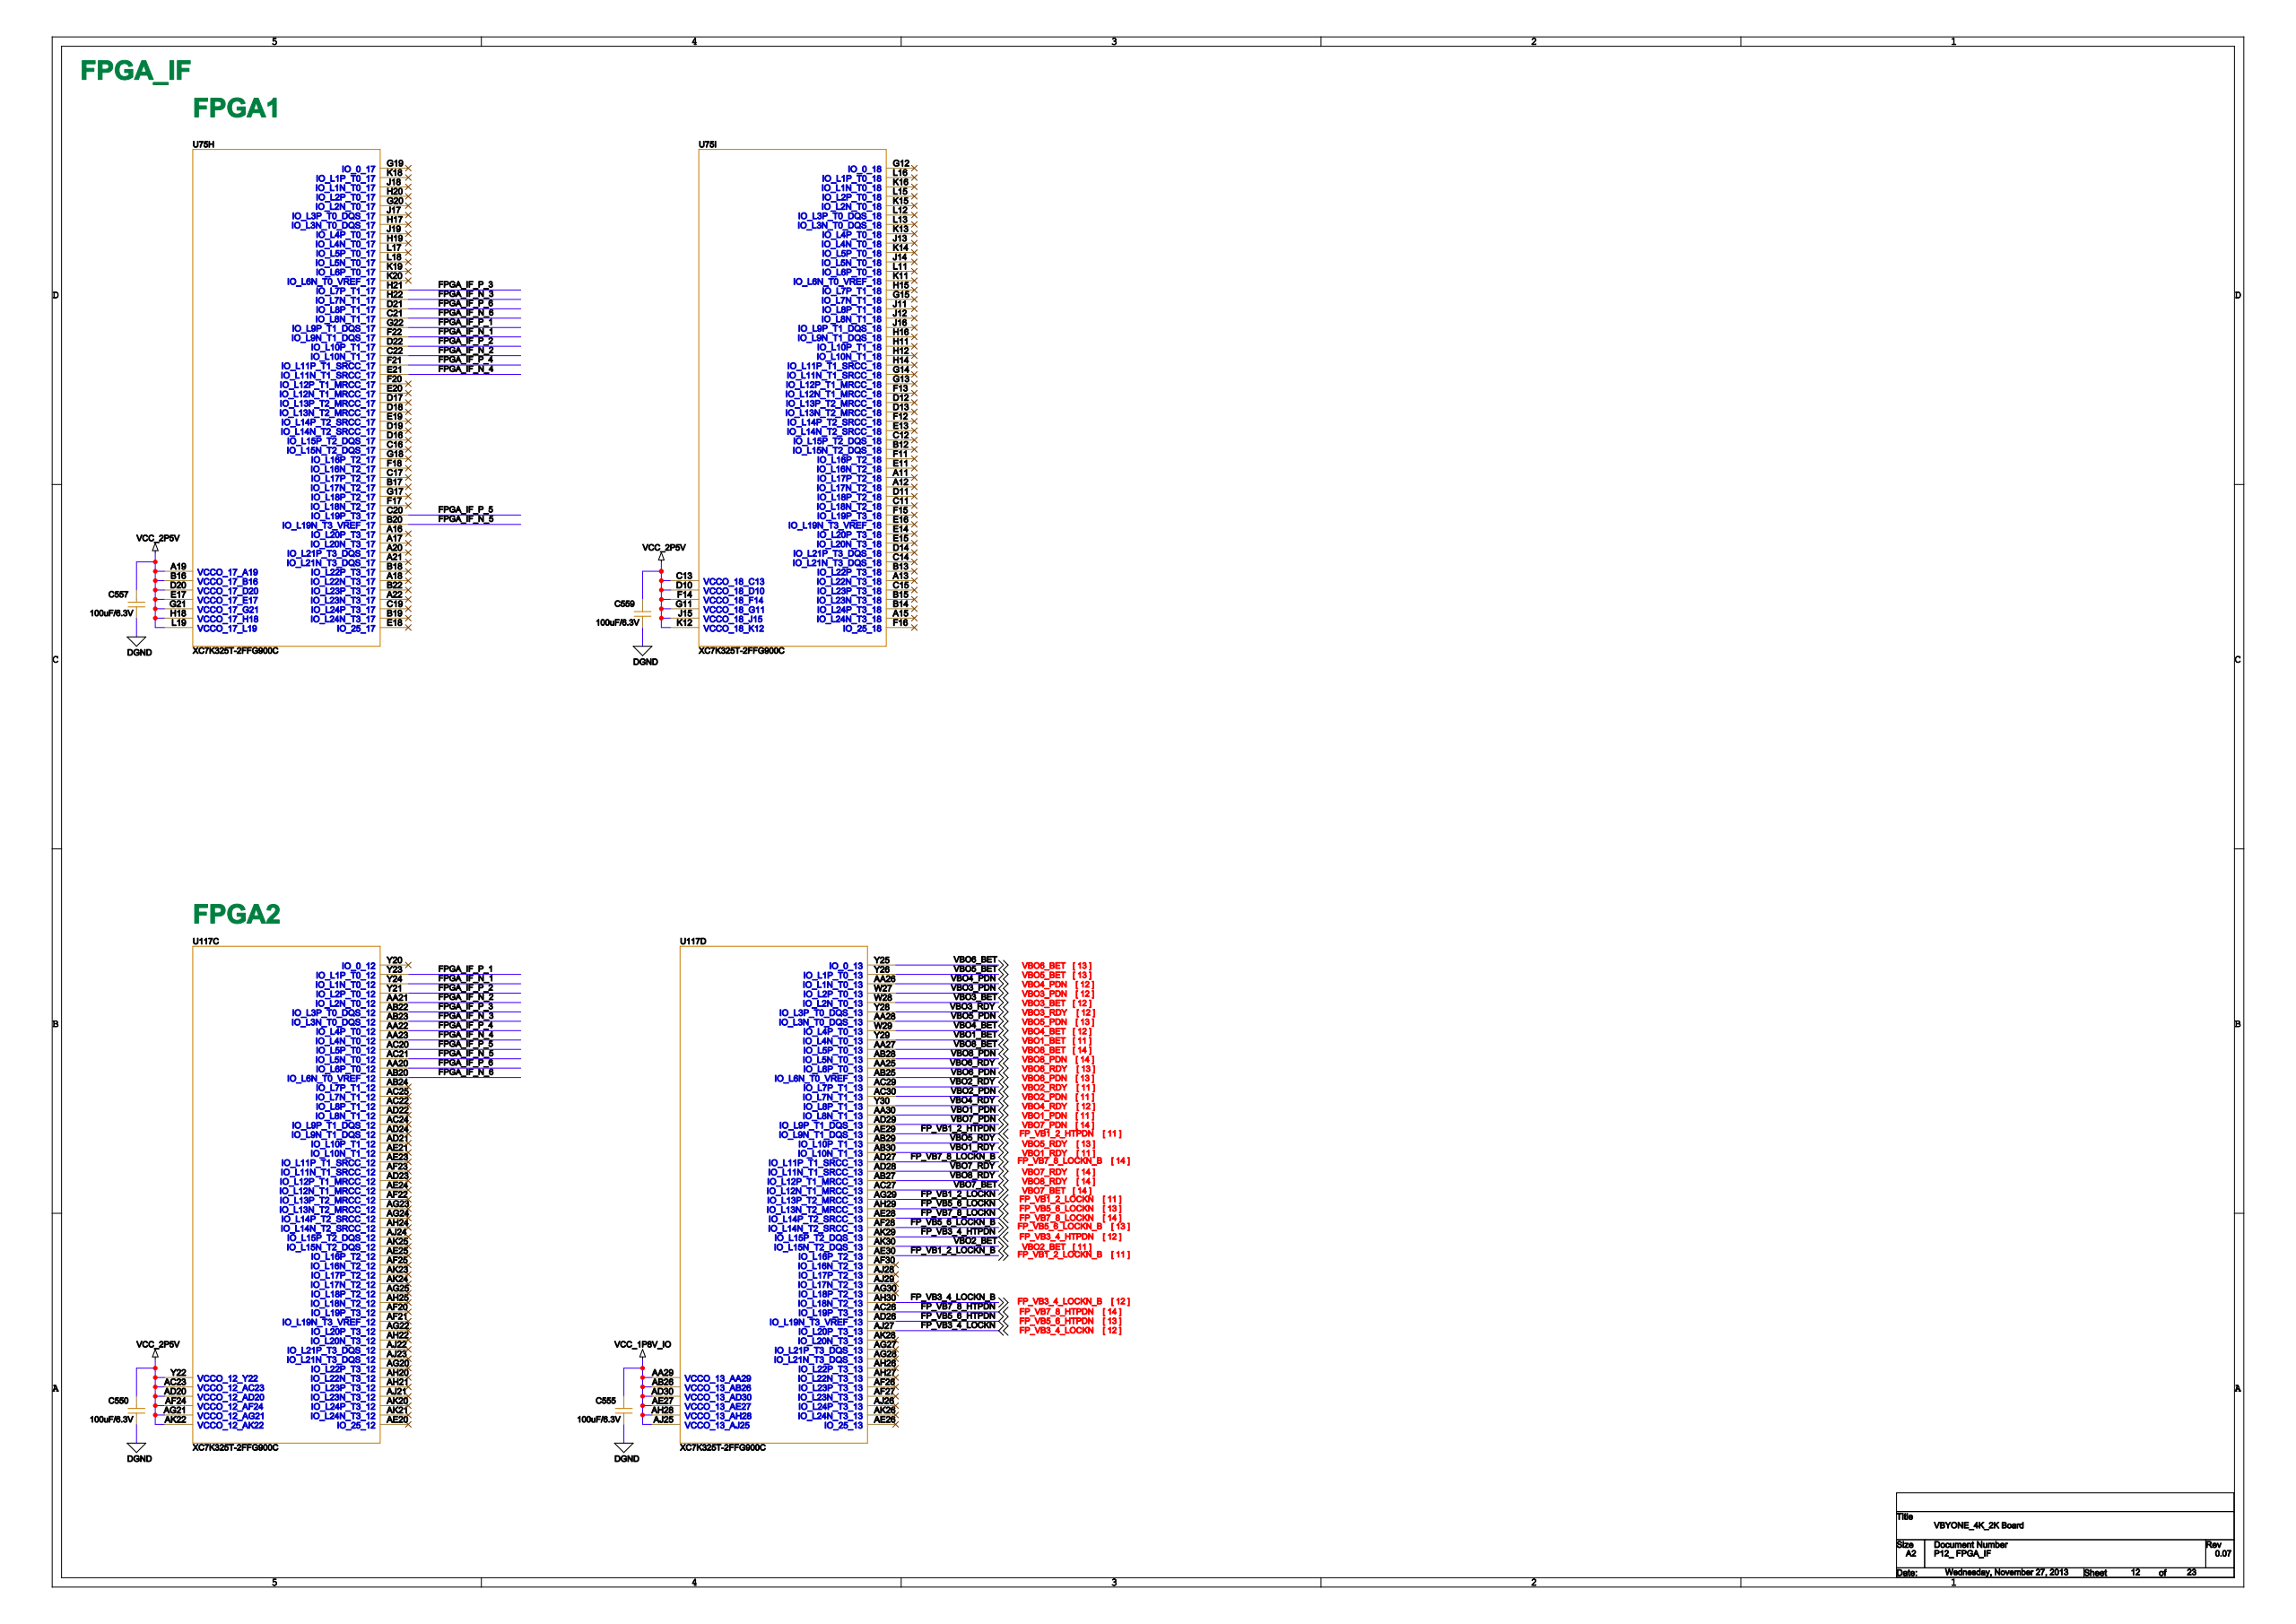Circuit board | Cadence Allegro | 1712 parts | 1495 nets | one sheet of the schematic
Parts on this sheet (reference | value | footprint):
C550 | 100uF/6.3V | CRC3225RZAS
C555 | 100uF/6.3V | CRC3225RZAS
C557 | 100uF/6.3V | CRC3225RZAS
C559 | 100uF/6.3V | CRC3225RZAS
U75 | XC7K325T-2FFG900C | BGA900RGAS
U117 | XC7K325T-2FFG900C | BGA900RGAS
Nets of these parts (net: part-pin ...):
DGND: C550-1 C555-1 C557-1 C559-1 U75-A2 U117-A2
VCC_2P5V: C550-2 C557-2 C559-2 U75-A19 U75-AA29 U75-AB26 U75-AC23 U75-AD20 U75-AD30 U75-AE27 U75-AF24 U75-AG21 U75-AH28 U75-AJ25 U75-AK22 U75-B16 U75-C13 U75-D10 U75-D20 U75-E17 U75-F14 U75-G11 U75-G21 U75-H18 U75-J15 U75-K12 U75-L19 U75-Y22 U117-A19 U117-AC23 U117-AD20 U117-AF24 U117-AG21 U117-AK22 U117-B16 U117-C13 U117-D10 U117-D20 U117-E17 U117-F14 U117-G11 U117-G21 U117-H18 U117-J15 U117-K12 U117-L19 U117-Y22
VCC_1P8V_IO: C555-2 U117-AA29 U117-AB26 U117-AD30 U117-AE27 U117-AH28 U117-AJ25
FP_VB7_8_HTPDN: U117-AC26
FP_VB7_8_LOCKN: U117-AE28
FP_VB7_8_LOCKN_B: U117-AD27
FP_VB1_2_HTPDN: U117-AE29
FP_VB1_2_LOCKN: U117-AG29
FP_VB1_2_LOCKN_B: U117-AE30
FP_VB3_4_HTPDN: U117-AK29
FP_VB3_4_LOCKN: U117-AJ27
FP_VB3_4_LOCKN_B: U117-AH30
FP_VB5_6_HTPDN: U117-AD26
FP_VB5_6_LOCKN: U117-AH29
FP_VB5_6_LOCKN_B: U117-AF28
VBO8_RDY: U117-AB27
VBO8_PDN: U117-AB28
VBO8_BET: U117-AA27
VBO1_RDY: U117-AB30
VBO1_PDN: U117-AA30
VBO1_BET: U117-Y29
VBO2_RDY: U117-AC29
VBO2_PDN: U117-AC30
VBO2_BET: U117-AK30
VBO3_RDY: U117-Y28
VBO3_PDN: U117-W27
VBO3_BET: U117-W28
VBO4_PDN: U117-AA26
VBO4_RDY: U117-Y30
VBO4_BET: U117-W29
VBO5_RDY: U117-AB29
VBO5_PDN: U117-AA28
VBO5_BET: U117-Y26
VBO6_PDN: U117-AB25
VBO6_RDY: U117-AA25
VBO6_BET: U117-Y25
VBO7_RDY: U117-AD28
VBO7_PDN: U117-AD29
VBO7_BET: U117-AC27
FPGA_IF_P_5: U75-C20 U117-AC20
FPGA_IF_N_6: U75-C21 U117-AB20
FPGA_IF_P_6: U75-D21 U117-AA20
FPGA_IF_N_5: U75-B20 U117-AC21
FPGA_IF_N_2: U75-C22 U117-AA21
FPGA_IF_P_2: U75-D22 U117-Y21
FPGA_IF_P_3: U75-H21 U117-AB22
FPGA_IF_P_4: U75-F21 U117-AA22
FPGA_IF_N_3: U75-H22 U117-AB23
FPGA_IF_N_4: U75-E21 U117-AA23
FPGA_IF_P_1: U75-G22 U117-Y23
FPGA_IF_N_1: U75-F22 U117-Y24